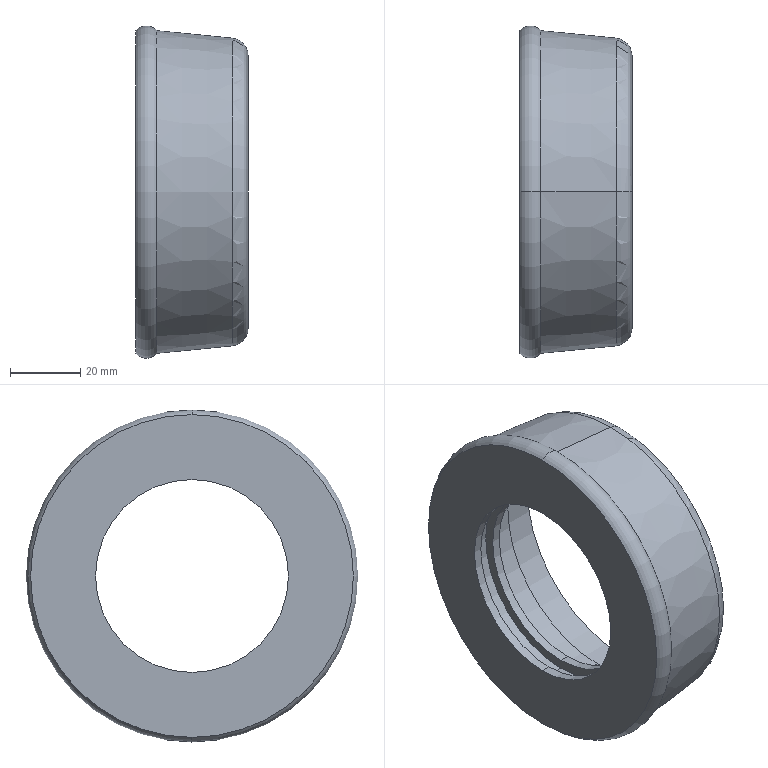Part | SolidWorks | features Revolution 1 | 1 solid | 22 faces | box 32 x 94.708 x 94.708 mm | volume 83187 mm3 | cylinder 10 | plane 6 | torus 4 | cone 2 | commonest cylinder face diameters 55 x4 60.7 x2 72 x2 76 x2
STEP:
#1=CARTESIAN_POINT('',(27.498,0.,43.85));
#2=VERTEX_POINT('',#1);
#3=CARTESIAN_POINT('',(27.498,0.,-43.85));
#4=VERTEX_POINT('',#3);
#5=CARTESIAN_POINT('',(27.498,0.,0.));
#6=DIRECTION('',(-1.,0.,0.));
#7=DIRECTION('',(0.,0.,1.));
#8=AXIS2_PLACEMENT_3D('',#5,#6,#7);
#9=CIRCLE('',#8,43.85);
#10=EDGE_CURVE('',#2,#4,#9,.T.);
#11=ORIENTED_EDGE('',*,*,#10,.T.);
#12=CARTESIAN_POINT('',(6.,0.,-46.));
#13=VERTEX_POINT('',#12);
#14=CARTESIAN_POINT('',(27.498,0.,-43.85));
#15=DIRECTION('',(-0.995,0.,-0.0995));
#16=VECTOR('',#15,1000.);
#17=LINE('',#14,#16);
#18=EDGE_CURVE('',#4,#13,#17,.T.);
#19=ORIENTED_EDGE('',*,*,#18,.T.);
#20=CARTESIAN_POINT('',(6.,0.,46.));
#21=VERTEX_POINT('',#20);
#22=CARTESIAN_POINT('',(6.,0.,0.));
#23=DIRECTION('',(-1.,0.,0.));
#24=DIRECTION('',(0.,0.,1.));
#25=AXIS2_PLACEMENT_3D('',#22,#23,#24);
#26=CIRCLE('',#25,46.);
#27=EDGE_CURVE('',#21,#13,#26,.T.);
#28=ORIENTED_EDGE('',*,*,#27,.F.);
#29=CARTESIAN_POINT('',(27.498,0.,43.85));
#30=DIRECTION('',(-0.995,0.,0.0995));
#31=VECTOR('',#30,1000.);
#32=LINE('',#29,#31);
#33=EDGE_CURVE('',#2,#21,#32,.T.);
#34=ORIENTED_EDGE('',*,*,#33,.F.);
#35=EDGE_LOOP('',(#11,#19,#28,#34));
#36=FACE_OUTER_BOUND('',#35,.T.);
#37=CARTESIAN_POINT('',(27.498,0.,0.));
#38=DIRECTION('',(-1.,0.,0.));
#39=DIRECTION('',(0.,0.,1.));
#40=AXIS2_PLACEMENT_3D('',#37,#38,#39);
#41=CONICAL_SURFACE('',#40,43.85,0.09967);
#42=ADVANCED_FACE('',(#36),#41,.T.);
#43=CARTESIAN_POINT('',(32.,0.,38.875));
#44=VERTEX_POINT('',#43);
#45=CARTESIAN_POINT('',(32.,0.,-38.875));
#46=VERTEX_POINT('',#45);
#47=CARTESIAN_POINT('',(32.,0.,0.));
#48=DIRECTION('',(-1.,0.,0.));
#49=DIRECTION('',(0.,0.,1.));
#50=AXIS2_PLACEMENT_3D('',#47,#48,#49);
#51=CIRCLE('',#50,38.875);
#52=EDGE_CURVE('',#44,#46,#51,.T.);
#53=ORIENTED_EDGE('',*,*,#52,.T.);
#54=CARTESIAN_POINT('',(27.,0.,-38.875));
#55=DIRECTION('',(0.,1.,0.));
#56=DIRECTION('',(0.,0.,1.));
#57=AXIS2_PLACEMENT_3D('',#54,#55,#56);
#58=CIRCLE('',#57,5.);
#59=EDGE_CURVE('',#46,#4,#58,.T.);
#60=ORIENTED_EDGE('',*,*,#59,.T.);
#61=ORIENTED_EDGE('',*,*,#10,.F.);
#62=CARTESIAN_POINT('',(27.,0.,38.875));
#63=DIRECTION('',(0.,-1.,0.));
#64=DIRECTION('',(0.,0.,-1.));
#65=AXIS2_PLACEMENT_3D('',#62,#63,#64);
#66=CIRCLE('',#65,5.);
#67=EDGE_CURVE('',#44,#2,#66,.T.);
#68=ORIENTED_EDGE('',*,*,#67,.F.);
#69=EDGE_LOOP('',(#53,#60,#61,#68));
#70=FACE_OUTER_BOUND('',#69,.T.);
#71=CARTESIAN_POINT('',(27.,0.,0.));
#72=DIRECTION('',(-1.,0.,0.));
#73=DIRECTION('',(0.,0.,1.));
#74=AXIS2_PLACEMENT_3D('',#71,#72,#73);
#75=TOROIDAL_SURFACE('',#74,38.875,5.);
#76=ADVANCED_FACE('',(#70),#75,.T.);
#77=CARTESIAN_POINT('',(32.,0.,-38.));
#78=VERTEX_POINT('',#77);
#79=CARTESIAN_POINT('',(32.,0.,38.));
#80=VERTEX_POINT('',#79);
#81=CARTESIAN_POINT('',(32.,0.,0.));
#82=DIRECTION('',(-1.,0.,0.));
#83=DIRECTION('',(0.,0.,1.));
#84=AXIS2_PLACEMENT_3D('',#81,#82,#83);
#85=CIRCLE('',#84,38.);
#86=EDGE_CURVE('',#78,#80,#85,.T.);
#87=ORIENTED_EDGE('',*,*,#86,.F.);
#88=CARTESIAN_POINT('',(22.,0.,-38.));
#89=VERTEX_POINT('',#88);
#90=CARTESIAN_POINT('',(-44.682,0.,-38.));
#91=DIRECTION('',(-1.,0.,0.));
#92=VECTOR('',#91,1000.);
#93=LINE('',#90,#92);
#94=EDGE_CURVE('',#78,#89,#93,.T.);
#95=ORIENTED_EDGE('',*,*,#94,.T.);
#96=CARTESIAN_POINT('',(22.,0.,38.));
#97=VERTEX_POINT('',#96);
#98=CARTESIAN_POINT('',(22.,0.,0.));
#99=DIRECTION('',(-1.,0.,0.));
#100=DIRECTION('',(0.,0.,1.));
#101=AXIS2_PLACEMENT_3D('',#98,#99,#100);
#102=CIRCLE('',#101,38.);
#103=EDGE_CURVE('',#89,#97,#102,.T.);
#104=ORIENTED_EDGE('',*,*,#103,.T.);
#105=CARTESIAN_POINT('',(-44.682,0.,38.));
#106=DIRECTION('',(-1.,0.,0.));
#107=VECTOR('',#106,1000.);
#108=LINE('',#105,#107);
#109=EDGE_CURVE('',#80,#97,#108,.T.);
#110=ORIENTED_EDGE('',*,*,#109,.F.);
#111=EDGE_LOOP('',(#87,#95,#104,#110));
#112=FACE_OUTER_BOUND('',#111,.T.);
#113=CARTESIAN_POINT('',(-44.682,0.,0.));
#114=DIRECTION('',(-1.,0.,0.));
#115=DIRECTION('',(0.,0.,1.));
#116=AXIS2_PLACEMENT_3D('',#113,#114,#115);
#117=CYLINDRICAL_SURFACE('',#116,38.);
#118=ADVANCED_FACE('',(#112),#117,.F.);
#119=CARTESIAN_POINT('',(22.,0.,-36.));
#120=VERTEX_POINT('',#119);
#121=CARTESIAN_POINT('',(22.,0.,36.));
#122=VERTEX_POINT('',#121);
#123=CARTESIAN_POINT('',(22.,0.,0.));
#124=DIRECTION('',(-1.,0.,0.));
#125=DIRECTION('',(0.,0.,1.));
#126=AXIS2_PLACEMENT_3D('',#123,#124,#125);
#127=CIRCLE('',#126,36.);
#128=EDGE_CURVE('',#120,#122,#127,.T.);
#129=ORIENTED_EDGE('',*,*,#128,.F.);
#130=CARTESIAN_POINT('',(10.,0.,-36.));
#131=VERTEX_POINT('',#130);
#132=CARTESIAN_POINT('',(-44.682,0.,-36.));
#133=DIRECTION('',(-1.,0.,0.));
#134=VECTOR('',#133,1000.);
#135=LINE('',#132,#134);
#136=EDGE_CURVE('',#120,#131,#135,.T.);
#137=ORIENTED_EDGE('',*,*,#136,.T.);
#138=CARTESIAN_POINT('',(10.,0.,36.));
#139=VERTEX_POINT('',#138);
#140=CARTESIAN_POINT('',(10.,0.,0.));
#141=DIRECTION('',(-1.,0.,0.));
#142=DIRECTION('',(0.,0.,1.));
#143=AXIS2_PLACEMENT_3D('',#140,#141,#142);
#144=CIRCLE('',#143,36.);
#145=EDGE_CURVE('',#131,#139,#144,.T.);
#146=ORIENTED_EDGE('',*,*,#145,.T.);
#147=CARTESIAN_POINT('',(-44.682,0.,36.));
#148=DIRECTION('',(-1.,0.,0.));
#149=VECTOR('',#148,1000.);
#150=LINE('',#147,#149);
#151=EDGE_CURVE('',#122,#139,#150,.T.);
#152=ORIENTED_EDGE('',*,*,#151,.F.);
#153=EDGE_LOOP('',(#129,#137,#146,#152));
#154=FACE_OUTER_BOUND('',#153,.T.);
#155=CARTESIAN_POINT('',(-44.682,0.,0.));
#156=DIRECTION('',(-1.,0.,0.));
#157=DIRECTION('',(0.,0.,1.));
#158=AXIS2_PLACEMENT_3D('',#155,#156,#157);
#159=CYLINDRICAL_SURFACE('',#158,36.);
#160=ADVANCED_FACE('',(#154),#159,.F.);
#161=CARTESIAN_POINT('',(10.,0.,-27.5));
#162=VERTEX_POINT('',#161);
#163=CARTESIAN_POINT('',(10.,0.,27.5));
#164=VERTEX_POINT('',#163);
#165=CARTESIAN_POINT('',(10.,0.,0.));
#166=DIRECTION('',(-1.,0.,0.));
#167=DIRECTION('',(0.,0.,1.));
#168=AXIS2_PLACEMENT_3D('',#165,#166,#167);
#169=CIRCLE('',#168,27.5);
#170=EDGE_CURVE('',#162,#164,#169,.T.);
#171=ORIENTED_EDGE('',*,*,#170,.F.);
#172=CARTESIAN_POINT('',(7.4,0.,-27.5));
#173=VERTEX_POINT('',#172);
#174=CARTESIAN_POINT('',(-44.682,0.,-27.5));
#175=DIRECTION('',(-1.,0.,0.));
#176=VECTOR('',#175,1000.);
#177=LINE('',#174,#176);
#178=EDGE_CURVE('',#162,#173,#177,.T.);
#179=ORIENTED_EDGE('',*,*,#178,.T.);
#180=CARTESIAN_POINT('',(7.4,0.,27.5));
#181=VERTEX_POINT('',#180);
#182=CARTESIAN_POINT('',(7.4,0.,0.));
#183=DIRECTION('',(-1.,0.,0.));
#184=DIRECTION('',(0.,0.,1.));
#185=AXIS2_PLACEMENT_3D('',#182,#183,#184);
#186=CIRCLE('',#185,27.5);
#187=EDGE_CURVE('',#173,#181,#186,.T.);
#188=ORIENTED_EDGE('',*,*,#187,.T.);
#189=CARTESIAN_POINT('',(-44.682,0.,27.5));
#190=DIRECTION('',(-1.,0.,0.));
#191=VECTOR('',#190,1000.);
#192=LINE('',#189,#191);
#193=EDGE_CURVE('',#164,#181,#192,.T.);
#194=ORIENTED_EDGE('',*,*,#193,.F.);
#195=EDGE_LOOP('',(#171,#179,#188,#194));
#196=FACE_OUTER_BOUND('',#195,.T.);
#197=CARTESIAN_POINT('',(-44.682,0.,0.));
#198=DIRECTION('',(-1.,0.,0.));
#199=DIRECTION('',(0.,0.,1.));
#200=AXIS2_PLACEMENT_3D('',#197,#198,#199);
#201=CYLINDRICAL_SURFACE('',#200,27.5);
#202=ADVANCED_FACE('',(#196),#201,.F.);
#203=CARTESIAN_POINT('',(7.4,0.,-30.35));
#204=VERTEX_POINT('',#203);
#205=CARTESIAN_POINT('',(7.4,0.,30.35));
#206=VERTEX_POINT('',#205);
#207=CARTESIAN_POINT('',(7.4,0.,0.));
#208=DIRECTION('',(-1.,0.,0.));
#209=DIRECTION('',(0.,0.,1.));
#210=AXIS2_PLACEMENT_3D('',#207,#208,#209);
#211=CIRCLE('',#210,30.35);
#212=EDGE_CURVE('',#204,#206,#211,.T.);
#213=ORIENTED_EDGE('',*,*,#212,.F.);
#214=CARTESIAN_POINT('',(2.6,0.,-30.35));
#215=VERTEX_POINT('',#214);
#216=CARTESIAN_POINT('',(-44.682,0.,-30.35));
#217=DIRECTION('',(-1.,0.,0.));
#218=VECTOR('',#217,1000.);
#219=LINE('',#216,#218);
#220=EDGE_CURVE('',#204,#215,#219,.T.);
#221=ORIENTED_EDGE('',*,*,#220,.T.);
#222=CARTESIAN_POINT('',(2.6,0.,30.35));
#223=VERTEX_POINT('',#222);
#224=CARTESIAN_POINT('',(2.6,0.,0.));
#225=DIRECTION('',(-1.,0.,0.));
#226=DIRECTION('',(0.,0.,1.));
#227=AXIS2_PLACEMENT_3D('',#224,#225,#226);
#228=CIRCLE('',#227,30.35);
#229=EDGE_CURVE('',#215,#223,#228,.T.);
#230=ORIENTED_EDGE('',*,*,#229,.T.);
#231=CARTESIAN_POINT('',(-44.682,0.,30.35));
#232=DIRECTION('',(-1.,0.,0.));
#233=VECTOR('',#232,1000.);
#234=LINE('',#231,#233);
#235=EDGE_CURVE('',#206,#223,#234,.T.);
#236=ORIENTED_EDGE('',*,*,#235,.F.);
#237=EDGE_LOOP('',(#213,#221,#230,#236));
#238=FACE_OUTER_BOUND('',#237,.T.);
#239=CARTESIAN_POINT('',(-44.682,0.,0.));
#240=DIRECTION('',(-1.,0.,0.));
#241=DIRECTION('',(0.,0.,1.));
#242=AXIS2_PLACEMENT_3D('',#239,#240,#241);
#243=CYLINDRICAL_SURFACE('',#242,30.35);
#244=ADVANCED_FACE('',(#238),#243,.F.);
#245=CARTESIAN_POINT('',(2.6,0.,-27.5));
#246=VERTEX_POINT('',#245);
#247=CARTESIAN_POINT('',(2.6,0.,27.5));
#248=VERTEX_POINT('',#247);
#249=CARTESIAN_POINT('',(2.6,0.,0.));
#250=DIRECTION('',(-1.,0.,0.));
#251=DIRECTION('',(0.,0.,1.));
#252=AXIS2_PLACEMENT_3D('',#249,#250,#251);
#253=CIRCLE('',#252,27.5);
#254=EDGE_CURVE('',#246,#248,#253,.T.);
#255=ORIENTED_EDGE('',*,*,#254,.F.);
#256=CARTESIAN_POINT('',(0.,0.,-27.5));
#257=VERTEX_POINT('',#256);
#258=CARTESIAN_POINT('',(-44.682,0.,-27.5));
#259=DIRECTION('',(-1.,0.,0.));
#260=VECTOR('',#259,1000.);
#261=LINE('',#258,#260);
#262=EDGE_CURVE('',#246,#257,#261,.T.);
#263=ORIENTED_EDGE('',*,*,#262,.T.);
#264=CARTESIAN_POINT('',(0.,0.,27.5));
#265=VERTEX_POINT('',#264);
#266=CARTESIAN_POINT('',(0.,0.,0.));
#267=DIRECTION('',(-1.,0.,0.));
#268=DIRECTION('',(0.,0.,1.));
#269=AXIS2_PLACEMENT_3D('',#266,#267,#268);
#270=CIRCLE('',#269,27.5);
#271=EDGE_CURVE('',#257,#265,#270,.T.);
#272=ORIENTED_EDGE('',*,*,#271,.T.);
#273=CARTESIAN_POINT('',(-44.682,0.,27.5));
#274=DIRECTION('',(-1.,0.,0.));
#275=VECTOR('',#274,1000.);
#276=LINE('',#273,#275);
#277=EDGE_CURVE('',#248,#265,#276,.T.);
#278=ORIENTED_EDGE('',*,*,#277,.F.);
#279=EDGE_LOOP('',(#255,#263,#272,#278));
#280=FACE_OUTER_BOUND('',#279,.T.);
#281=CARTESIAN_POINT('',(-44.682,0.,0.));
#282=DIRECTION('',(-1.,0.,0.));
#283=DIRECTION('',(0.,0.,1.));
#284=AXIS2_PLACEMENT_3D('',#281,#282,#283);
#285=CYLINDRICAL_SURFACE('',#284,27.5);
#286=ADVANCED_FACE('',(#280),#285,.F.);
#287=ORIENTED_EDGE('',*,*,#27,.T.);
#288=CARTESIAN_POINT('',(0.,0.,-46.));
#289=VERTEX_POINT('',#288);
#290=CARTESIAN_POINT('',(3.,0.,-43.354));
#291=DIRECTION('',(0.,1.,0.));
#292=DIRECTION('',(0.,0.,1.));
#293=AXIS2_PLACEMENT_3D('',#290,#291,#292);
#294=CIRCLE('',#293,4.);
#295=EDGE_CURVE('',#13,#289,#294,.T.);
#296=ORIENTED_EDGE('',*,*,#295,.T.);
#297=CARTESIAN_POINT('',(0.,0.,46.));
#298=VERTEX_POINT('',#297);
#299=CARTESIAN_POINT('',(0.,0.,0.));
#300=DIRECTION('',(-1.,0.,0.));
#301=DIRECTION('',(0.,0.,1.));
#302=AXIS2_PLACEMENT_3D('',#299,#300,#301);
#303=CIRCLE('',#302,46.);
#304=EDGE_CURVE('',#298,#289,#303,.T.);
#305=ORIENTED_EDGE('',*,*,#304,.F.);
#306=CARTESIAN_POINT('',(3.,0.,43.354));
#307=DIRECTION('',(0.,-1.,0.));
#308=DIRECTION('',(0.,0.,-1.));
#309=AXIS2_PLACEMENT_3D('',#306,#307,#308);
#310=CIRCLE('',#309,4.);
#311=EDGE_CURVE('',#21,#298,#310,.T.);
#312=ORIENTED_EDGE('',*,*,#311,.F.);
#313=EDGE_LOOP('',(#287,#296,#305,#312));
#314=FACE_OUTER_BOUND('',#313,.T.);
#315=CARTESIAN_POINT('',(3.,0.,0.));
#316=DIRECTION('',(-1.,0.,0.));
#317=DIRECTION('',(0.,0.,1.));
#318=AXIS2_PLACEMENT_3D('',#315,#316,#317);
#319=TOROIDAL_SURFACE('',#318,43.354,4.);
#320=ADVANCED_FACE('',(#314),#319,.T.);
#321=ORIENTED_EDGE('',*,*,#295,.F.);
#322=CARTESIAN_POINT('',(6.,0.,0.));
#323=DIRECTION('',(-1.,0.,0.));
#324=DIRECTION('',(0.,0.,1.));
#325=AXIS2_PLACEMENT_3D('',#322,#323,#324);
#326=CIRCLE('',#325,46.);
#327=EDGE_CURVE('',#13,#21,#326,.T.);
#328=ORIENTED_EDGE('',*,*,#327,.T.);
#329=ORIENTED_EDGE('',*,*,#311,.T.);
#330=CARTESIAN_POINT('',(0.,0.,0.));
#331=DIRECTION('',(-1.,0.,0.));
#332=DIRECTION('',(0.,0.,1.));
#333=AXIS2_PLACEMENT_3D('',#330,#331,#332);
#334=CIRCLE('',#333,46.);
#335=EDGE_CURVE('',#289,#298,#334,.T.);
#336=ORIENTED_EDGE('',*,*,#335,.F.);
#337=EDGE_LOOP('',(#321,#328,#329,#336));
#338=FACE_OUTER_BOUND('',#337,.T.);
#339=CARTESIAN_POINT('',(3.,0.,0.));
#340=DIRECTION('',(-1.,0.,0.));
#341=DIRECTION('',(0.,0.,1.));
#342=AXIS2_PLACEMENT_3D('',#339,#340,#341);
#343=TOROIDAL_SURFACE('',#342,43.354,4.);
#344=ADVANCED_FACE('',(#338),#343,.T.);
#345=CARTESIAN_POINT('',(0.,0.,0.));
#346=DIRECTION('',(-1.,0.,0.));
#347=DIRECTION('',(0.,0.,1.));
#348=AXIS2_PLACEMENT_3D('',#345,#346,#347);
#349=CIRCLE('',#348,27.5);
#350=EDGE_CURVE('',#265,#257,#349,.T.);
#351=ORIENTED_EDGE('',*,*,#350,.F.);
#352=ORIENTED_EDGE('',*,*,#271,.F.);
#353=EDGE_LOOP('',(#351,#352));
#354=FACE_BOUND('',#353,.T.);
#355=ORIENTED_EDGE('',*,*,#304,.T.);
#356=ORIENTED_EDGE('',*,*,#335,.T.);
#357=EDGE_LOOP('',(#355,#356));
#358=FACE_OUTER_BOUND('',#357,.T.);
#359=CARTESIAN_POINT('',(0.,27.5,0.));
#360=DIRECTION('',(1.,0.,0.));
#361=DIRECTION('',(0.,0.,-1.));
#362=AXIS2_PLACEMENT_3D('',#359,#360,#361);
#363=PLANE('',#362);
#364=ADVANCED_FACE('',(#354,#358),#363,.F.);
#365=ORIENTED_EDGE('',*,*,#262,.F.);
#366=CARTESIAN_POINT('',(2.6,0.,0.));
#367=DIRECTION('',(-1.,0.,0.));
#368=DIRECTION('',(0.,0.,1.));
#369=AXIS2_PLACEMENT_3D('',#366,#367,#368);
#370=CIRCLE('',#369,27.5);
#371=EDGE_CURVE('',#248,#246,#370,.T.);
#372=ORIENTED_EDGE('',*,*,#371,.F.);
#373=ORIENTED_EDGE('',*,*,#277,.T.);
#374=ORIENTED_EDGE('',*,*,#350,.T.);
#375=EDGE_LOOP('',(#365,#372,#373,#374));
#376=FACE_OUTER_BOUND('',#375,.T.);
#377=CARTESIAN_POINT('',(-44.682,0.,0.));
#378=DIRECTION('',(-1.,0.,0.));
#379=DIRECTION('',(0.,0.,1.));
#380=AXIS2_PLACEMENT_3D('',#377,#378,#379);
#381=CYLINDRICAL_SURFACE('',#380,27.5);
#382=ADVANCED_FACE('',(#376),#381,.F.);
#383=CARTESIAN_POINT('',(2.6,0.,0.));
#384=DIRECTION('',(-1.,0.,0.));
#385=DIRECTION('',(0.,0.,1.));
#386=AXIS2_PLACEMENT_3D('',#383,#384,#385);
#387=CIRCLE('',#386,30.35);
#388=EDGE_CURVE('',#223,#215,#387,.T.);
#389=ORIENTED_EDGE('',*,*,#388,.F.);
#390=ORIENTED_EDGE('',*,*,#229,.F.);
#391=EDGE_LOOP('',(#389,#390));
#392=FACE_OUTER_BOUND('',#391,.T.);
#393=ORIENTED_EDGE('',*,*,#371,.T.);
#394=ORIENTED_EDGE('',*,*,#254,.T.);
#395=EDGE_LOOP('',(#393,#394));
#396=FACE_BOUND('',#395,.T.);
#397=CARTESIAN_POINT('',(2.6,30.35,0.));
#398=DIRECTION('',(-1.,0.,0.));
#399=DIRECTION('',(0.,0.,1.));
#400=AXIS2_PLACEMENT_3D('',#397,#398,#399);
#401=PLANE('',#400);
#402=ADVANCED_FACE('',(#392,#396),#401,.F.);
#403=ORIENTED_EDGE('',*,*,#220,.F.);
#404=CARTESIAN_POINT('',(7.4,0.,0.));
#405=DIRECTION('',(-1.,0.,0.));
#406=DIRECTION('',(0.,0.,1.));
#407=AXIS2_PLACEMENT_3D('',#404,#405,#406);
#408=CIRCLE('',#407,30.35);
#409=EDGE_CURVE('',#206,#204,#408,.T.);
#410=ORIENTED_EDGE('',*,*,#409,.F.);
#411=ORIENTED_EDGE('',*,*,#235,.T.);
#412=ORIENTED_EDGE('',*,*,#388,.T.);
#413=EDGE_LOOP('',(#403,#410,#411,#412));
#414=FACE_OUTER_BOUND('',#413,.T.);
#415=CARTESIAN_POINT('',(-44.682,0.,0.));
#416=DIRECTION('',(-1.,0.,0.));
#417=DIRECTION('',(0.,0.,1.));
#418=AXIS2_PLACEMENT_3D('',#415,#416,#417);
#419=CYLINDRICAL_SURFACE('',#418,30.35);
#420=ADVANCED_FACE('',(#414),#419,.F.);
#421=CARTESIAN_POINT('',(7.4,0.,0.));
#422=DIRECTION('',(-1.,0.,0.));
#423=DIRECTION('',(0.,0.,1.));
#424=AXIS2_PLACEMENT_3D('',#421,#422,#423);
#425=CIRCLE('',#424,27.5);
#426=EDGE_CURVE('',#181,#173,#425,.T.);
#427=ORIENTED_EDGE('',*,*,#426,.F.);
#428=ORIENTED_EDGE('',*,*,#187,.F.);
#429=EDGE_LOOP('',(#427,#428));
#430=FACE_BOUND('',#429,.T.);
#431=ORIENTED_EDGE('',*,*,#409,.T.);
#432=ORIENTED_EDGE('',*,*,#212,.T.);
#433=EDGE_LOOP('',(#431,#432));
#434=FACE_OUTER_BOUND('',#433,.T.);
#435=CARTESIAN_POINT('',(7.4,30.35,0.));
#436=DIRECTION('',(1.,0.,0.));
#437=DIRECTION('',(0.,0.,-1.));
#438=AXIS2_PLACEMENT_3D('',#435,#436,#437);
#439=PLANE('',#438);
#440=ADVANCED_FACE('',(#430,#434),#439,.F.);
#441=ORIENTED_EDGE('',*,*,#178,.F.);
#442=CARTESIAN_POINT('',(10.,0.,0.));
#443=DIRECTION('',(-1.,0.,0.));
#444=DIRECTION('',(0.,0.,1.));
#445=AXIS2_PLACEMENT_3D('',#442,#443,#444);
#446=CIRCLE('',#445,27.5);
#447=EDGE_CURVE('',#164,#162,#446,.T.);
#448=ORIENTED_EDGE('',*,*,#447,.F.);
#449=ORIENTED_EDGE('',*,*,#193,.T.);
#450=ORIENTED_EDGE('',*,*,#426,.T.);
#451=EDGE_LOOP('',(#441,#448,#449,#450));
#452=FACE_OUTER_BOUND('',#451,.T.);
#453=CARTESIAN_POINT('',(-44.682,0.,0.));
#454=DIRECTION('',(-1.,0.,0.));
#455=DIRECTION('',(0.,0.,1.));
#456=AXIS2_PLACEMENT_3D('',#453,#454,#455);
#457=CYLINDRICAL_SURFACE('',#456,27.5);
#458=ADVANCED_FACE('',(#452),#457,.F.);
#459=CARTESIAN_POINT('',(10.,0.,0.));
#460=DIRECTION('',(-1.,0.,0.));
#461=DIRECTION('',(0.,0.,1.));
#462=AXIS2_PLACEMENT_3D('',#459,#460,#461);
#463=CIRCLE('',#462,36.);
#464=EDGE_CURVE('',#139,#131,#463,.T.);
#465=ORIENTED_EDGE('',*,*,#464,.F.);
#466=ORIENTED_EDGE('',*,*,#145,.F.);
#467=EDGE_LOOP('',(#465,#466));
#468=FACE_OUTER_BOUND('',#467,.T.);
#469=ORIENTED_EDGE('',*,*,#447,.T.);
#470=ORIENTED_EDGE('',*,*,#170,.T.);
#471=EDGE_LOOP('',(#469,#470));
#472=FACE_BOUND('',#471,.T.);
#473=CARTESIAN_POINT('',(10.,36.,0.));
#474=DIRECTION('',(-1.,0.,0.));
#475=DIRECTION('',(0.,0.,1.));
#476=AXIS2_PLACEMENT_3D('',#473,#474,#475);
#477=PLANE('',#476);
#478=ADVANCED_FACE('',(#468,#472),#477,.F.);
#479=ORIENTED_EDGE('',*,*,#136,.F.);
#480=CARTESIAN_POINT('',(22.,0.,0.));
#481=DIRECTION('',(-1.,0.,0.));
#482=DIRECTION('',(0.,0.,1.));
#483=AXIS2_PLACEMENT_3D('',#480,#481,#482);
#484=CIRCLE('',#483,36.);
#485=EDGE_CURVE('',#122,#120,#484,.T.);
#486=ORIENTED_EDGE('',*,*,#485,.F.);
#487=ORIENTED_EDGE('',*,*,#151,.T.);
#488=ORIENTED_EDGE('',*,*,#464,.T.);
#489=EDGE_LOOP('',(#479,#486,#487,#488));
#490=FACE_OUTER_BOUND('',#489,.T.);
#491=CARTESIAN_POINT('',(-44.682,0.,0.));
#492=DIRECTION('',(-1.,0.,0.));
#493=DIRECTION('',(0.,0.,1.));
#494=AXIS2_PLACEMENT_3D('',#491,#492,#493);
#495=CYLINDRICAL_SURFACE('',#494,36.);
#496=ADVANCED_FACE('',(#490),#495,.F.);
#497=CARTESIAN_POINT('',(22.,0.,0.));
#498=DIRECTION('',(-1.,0.,0.));
#499=DIRECTION('',(0.,0.,1.));
#500=AXIS2_PLACEMENT_3D('',#497,#498,#499);
#501=CIRCLE('',#500,38.);
#502=EDGE_CURVE('',#97,#89,#501,.T.);
#503=ORIENTED_EDGE('',*,*,#502,.F.);
#504=ORIENTED_EDGE('',*,*,#103,.F.);
#505=EDGE_LOOP('',(#503,#504));
#506=FACE_OUTER_BOUND('',#505,.T.);
#507=ORIENTED_EDGE('',*,*,#485,.T.);
#508=ORIENTED_EDGE('',*,*,#128,.T.);
#509=EDGE_LOOP('',(#507,#508));
#510=FACE_BOUND('',#509,.T.);
#511=CARTESIAN_POINT('',(22.,38.,0.));
#512=DIRECTION('',(-1.,0.,0.));
#513=DIRECTION('',(0.,0.,1.));
#514=AXIS2_PLACEMENT_3D('',#511,#512,#513);
#515=PLANE('',#514);
#516=ADVANCED_FACE('',(#506,#510),#515,.F.);
#517=ORIENTED_EDGE('',*,*,#94,.F.);
#518=CARTESIAN_POINT('',(32.,0.,0.));
#519=DIRECTION('',(-1.,0.,0.));
#520=DIRECTION('',(0.,0.,1.));
#521=AXIS2_PLACEMENT_3D('',#518,#519,#520);
#522=CIRCLE('',#521,38.);
#523=EDGE_CURVE('',#80,#78,#522,.T.);
#524=ORIENTED_EDGE('',*,*,#523,.F.);
#525=ORIENTED_EDGE('',*,*,#109,.T.);
#526=ORIENTED_EDGE('',*,*,#502,.T.);
#527=EDGE_LOOP('',(#517,#524,#525,#526));
#528=FACE_OUTER_BOUND('',#527,.T.);
#529=CARTESIAN_POINT('',(-44.682,0.,0.));
#530=DIRECTION('',(-1.,0.,0.));
#531=DIRECTION('',(0.,0.,1.));
#532=AXIS2_PLACEMENT_3D('',#529,#530,#531);
#533=CYLINDRICAL_SURFACE('',#532,38.);
#534=ADVANCED_FACE('',(#528),#533,.F.);
#535=ORIENTED_EDGE('',*,*,#52,.F.);
#536=CARTESIAN_POINT('',(32.,0.,0.));
#537=DIRECTION('',(-1.,0.,0.));
#538=DIRECTION('',(0.,0.,1.));
#539=AXIS2_PLACEMENT_3D('',#536,#537,#538);
#540=CIRCLE('',#539,38.875);
#541=EDGE_CURVE('',#46,#44,#540,.T.);
#542=ORIENTED_EDGE('',*,*,#541,.F.);
#543=EDGE_LOOP('',(#535,#542));
#544=FACE_OUTER_BOUND('',#543,.T.);
#545=ORIENTED_EDGE('',*,*,#523,.T.);
#546=ORIENTED_EDGE('',*,*,#86,.T.);
#547=EDGE_LOOP('',(#545,#546));
#548=FACE_BOUND('',#547,.T.);
#549=CARTESIAN_POINT('',(32.,38.875,0.));
#550=DIRECTION('',(-1.,0.,0.));
#551=DIRECTION('',(0.,0.,1.));
#552=AXIS2_PLACEMENT_3D('',#549,#550,#551);
#553=PLANE('',#552);
#554=ADVANCED_FACE('',(#544,#548),#553,.F.);
#555=ORIENTED_EDGE('',*,*,#59,.F.);
#556=ORIENTED_EDGE('',*,*,#541,.T.);
#557=ORIENTED_EDGE('',*,*,#67,.T.);
#558=CARTESIAN_POINT('',(27.498,0.,0.));
#559=DIRECTION('',(-1.,0.,0.));
#560=DIRECTION('',(0.,0.,1.));
#561=AXIS2_PLACEMENT_3D('',#558,#559,#560);
#562=CIRCLE('',#561,43.85);
#563=EDGE_CURVE('',#4,#2,#562,.T.);
#564=ORIENTED_EDGE('',*,*,#563,.F.);
#565=EDGE_LOOP('',(#555,#556,#557,#564));
#566=FACE_OUTER_BOUND('',#565,.T.);
#567=CARTESIAN_POINT('',(27.,0.,0.));
#568=DIRECTION('',(-1.,0.,0.));
#569=DIRECTION('',(0.,0.,1.));
#570=AXIS2_PLACEMENT_3D('',#567,#568,#569);
#571=TOROIDAL_SURFACE('',#570,38.875,5.);
#572=ADVANCED_FACE('',(#566),#571,.T.);
#573=ORIENTED_EDGE('',*,*,#18,.F.);
#574=ORIENTED_EDGE('',*,*,#563,.T.);
#575=ORIENTED_EDGE('',*,*,#33,.T.);
#576=ORIENTED_EDGE('',*,*,#327,.F.);
#577=EDGE_LOOP('',(#573,#574,#575,#576));
#578=FACE_OUTER_BOUND('',#577,.T.);
#579=CARTESIAN_POINT('',(27.498,0.,0.));
#580=DIRECTION('',(-1.,0.,0.));
#581=DIRECTION('',(0.,0.,1.));
#582=AXIS2_PLACEMENT_3D('',#579,#580,#581);
#583=CONICAL_SURFACE('',#582,43.85,0.09967);
#584=ADVANCED_FACE('',(#578),#583,.T.);
#585=CLOSED_SHELL('',(#42,#76,#118,#160,#202,#244,#286,#320,#344,#364,#382,#402,#420,#440,#458,#478,#496,#516,#534,#554,#572,#584));
#586=MANIFOLD_SOLID_BREP('',#585);
#587=CARTESIAN_POINT('',(0.,0.,0.));
#588=DIRECTION('',(0.,0.,1.));
#589=DIRECTION('',(1.,0.,0.));
#590=AXIS2_PLACEMENT_3D('',#587,#588,#589);
#591=(LENGTH_UNIT()NAMED_UNIT(*)SI_UNIT(.MILLI.,.METRE.));
#592=UNCERTAINTY_MEASURE_WITH_UNIT(LENGTH_MEASURE(0.00001),#591,'','');
#593=(NAMED_UNIT(*)PLANE_ANGLE_UNIT()SI_UNIT($,.RADIAN.));
#594=(NAMED_UNIT(*)SI_UNIT($,.STERADIAN.)SOLID_ANGLE_UNIT());
#595=(GEOMETRIC_REPRESENTATION_CONTEXT(3)GLOBAL_UNCERTAINTY_ASSIGNED_CONTEXT((#592))GLOBAL_UNIT_ASSIGNED_CONTEXT((#591,#593,#594))REPRESENTATION_CONTEXT('',''));
#596=ADVANCED_BREP_SHAPE_REPRESENTATION('',(#586,#590),#595);